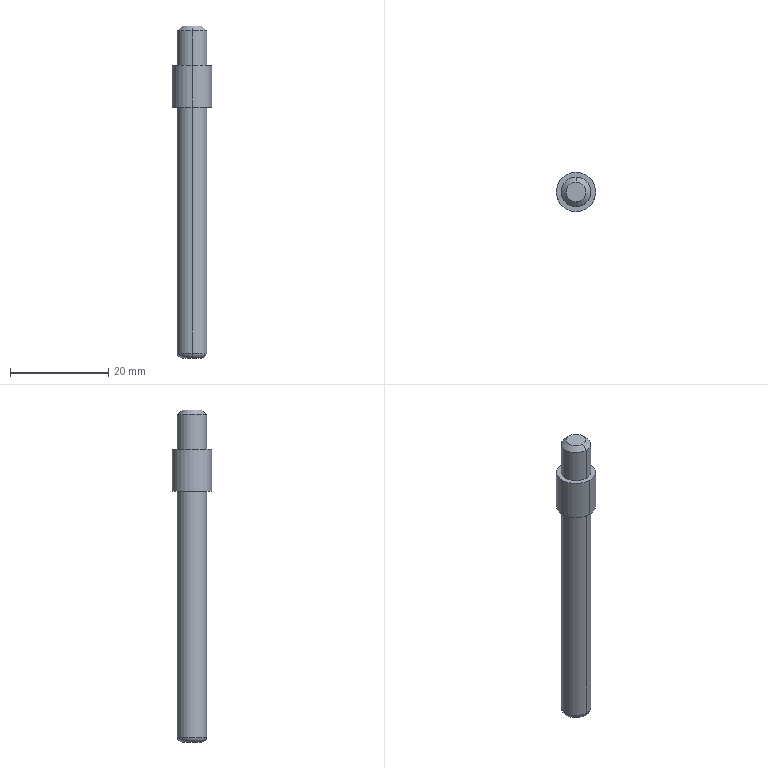Part | SolidWorks | features Chamfer 1, Fillet 1, Revolution 1 | 1 solid | 14 faces | box 8 x 8 x 67.5 mm | volume 2083 mm3 | cylinder 6 | plane 4 | cone 2 | torus 2 | commonest cylinder face diameters 6 x4 8 x2
STEP:
#1=CARTESIAN_POINT('',(0.,-2.,0.));
#2=VERTEX_POINT('',#1);
#3=CARTESIAN_POINT('',(0.,2.,0.));
#4=VERTEX_POINT('',#3);
#5=CARTESIAN_POINT('',(0.,0.,0.));
#6=DIRECTION('',(0.,0.,1.));
#7=DIRECTION('',(0.,-1.,0.));
#8=AXIS2_PLACEMENT_3D('',#5,#6,#7);
#9=CIRCLE('',#8,2.);
#10=EDGE_CURVE('',#2,#4,#9,.T.);
#11=ORIENTED_EDGE('',*,*,#10,.F.);
#12=CARTESIAN_POINT('',(0.,-3.,-1.));
#13=VERTEX_POINT('',#12);
#14=CARTESIAN_POINT('',(0.,-3.,-1.));
#15=DIRECTION('',(0.,-0.7071,-0.7071));
#16=VECTOR('',#15,1000.);
#17=LINE('',#14,#16);
#18=EDGE_CURVE('',#2,#13,#17,.T.);
#19=ORIENTED_EDGE('',*,*,#18,.T.);
#20=CARTESIAN_POINT('',(0.,3.,-1.));
#21=VERTEX_POINT('',#20);
#22=CARTESIAN_POINT('',(0.,0.,-1.));
#23=DIRECTION('',(0.,0.,-1.));
#24=DIRECTION('',(0.,-1.,0.));
#25=AXIS2_PLACEMENT_3D('',#22,#23,#24);
#26=CIRCLE('',#25,3.);
#27=EDGE_CURVE('',#21,#13,#26,.T.);
#28=ORIENTED_EDGE('',*,*,#27,.F.);
#29=CARTESIAN_POINT('',(0.,3.,-1.));
#30=DIRECTION('',(0.,0.7071,-0.7071));
#31=VECTOR('',#30,1000.);
#32=LINE('',#29,#31);
#33=EDGE_CURVE('',#4,#21,#32,.T.);
#34=ORIENTED_EDGE('',*,*,#33,.F.);
#35=EDGE_LOOP('',(#11,#19,#28,#34));
#36=FACE_OUTER_BOUND('',#35,.T.);
#37=CARTESIAN_POINT('',(0.,0.,-1.));
#38=DIRECTION('',(0.,0.,-1.));
#39=DIRECTION('',(0.,1.,0.));
#40=AXIS2_PLACEMENT_3D('',#37,#38,#39);
#41=CONICAL_SURFACE('',#40,3.,0.7854);
#42=ADVANCED_FACE('',(#36),#41,.T.);
#43=CARTESIAN_POINT('',(0.,-3.,-66.5));
#44=VERTEX_POINT('',#43);
#45=CARTESIAN_POINT('',(0.,3.,-66.5));
#46=VERTEX_POINT('',#45);
#47=CARTESIAN_POINT('',(0.,0.,-66.5));
#48=DIRECTION('',(0.,0.,1.));
#49=DIRECTION('',(0.,1.,0.));
#50=AXIS2_PLACEMENT_3D('',#47,#48,#49);
#51=CIRCLE('',#50,3.);
#52=EDGE_CURVE('',#44,#46,#51,.T.);
#53=ORIENTED_EDGE('',*,*,#52,.F.);
#54=CARTESIAN_POINT('',(0.,-2.,-67.5));
#55=VERTEX_POINT('',#54);
#56=CARTESIAN_POINT('',(0.,-2.,-66.5));
#57=DIRECTION('',(1.,0.,0.));
#58=DIRECTION('',(0.,1.,0.));
#59=AXIS2_PLACEMENT_3D('',#56,#57,#58);
#60=CIRCLE('',#59,1.);
#61=EDGE_CURVE('',#44,#55,#60,.T.);
#62=ORIENTED_EDGE('',*,*,#61,.T.);
#63=CARTESIAN_POINT('',(0.,2.,-67.5));
#64=VERTEX_POINT('',#63);
#65=CARTESIAN_POINT('',(0.,0.,-67.5));
#66=DIRECTION('',(0.,0.,-1.));
#67=DIRECTION('',(0.,1.,0.));
#68=AXIS2_PLACEMENT_3D('',#65,#66,#67);
#69=CIRCLE('',#68,2.);
#70=EDGE_CURVE('',#64,#55,#69,.T.);
#71=ORIENTED_EDGE('',*,*,#70,.F.);
#72=CARTESIAN_POINT('',(0.,2.,-66.5));
#73=DIRECTION('',(-1.,0.,0.));
#74=DIRECTION('',(0.,0.,1.));
#75=AXIS2_PLACEMENT_3D('',#72,#73,#74);
#76=CIRCLE('',#75,1.);
#77=EDGE_CURVE('',#46,#64,#76,.T.);
#78=ORIENTED_EDGE('',*,*,#77,.F.);
#79=EDGE_LOOP('',(#53,#62,#71,#78));
#80=FACE_OUTER_BOUND('',#79,.T.);
#81=CARTESIAN_POINT('',(0.,0.,-66.5));
#82=DIRECTION('',(0.,0.,-1.));
#83=DIRECTION('',(0.,1.,0.));
#84=AXIS2_PLACEMENT_3D('',#81,#82,#83);
#85=TOROIDAL_SURFACE('',#84,2.,1.);
#86=ADVANCED_FACE('',(#80),#85,.T.);
#87=CARTESIAN_POINT('',(0.,3.,-16.5));
#88=VERTEX_POINT('',#87);
#89=CARTESIAN_POINT('',(0.,-3.,-16.5));
#90=VERTEX_POINT('',#89);
#91=CARTESIAN_POINT('',(0.,0.,-16.5));
#92=DIRECTION('',(0.,0.,-1.));
#93=DIRECTION('',(0.,1.,0.));
#94=AXIS2_PLACEMENT_3D('',#91,#92,#93);
#95=CIRCLE('',#94,3.);
#96=EDGE_CURVE('',#88,#90,#95,.T.);
#97=ORIENTED_EDGE('',*,*,#96,.T.);
#98=CARTESIAN_POINT('',(0.,-3.,-67.5));
#99=DIRECTION('',(0.,0.,-1.));
#100=VECTOR('',#99,1000.);
#101=LINE('',#98,#100);
#102=EDGE_CURVE('',#90,#44,#101,.T.);
#103=ORIENTED_EDGE('',*,*,#102,.T.);
#104=ORIENTED_EDGE('',*,*,#52,.T.);
#105=CARTESIAN_POINT('',(0.,3.,-67.5));
#106=DIRECTION('',(0.,0.,-1.));
#107=VECTOR('',#106,1000.);
#108=LINE('',#105,#107);
#109=EDGE_CURVE('',#88,#46,#108,.T.);
#110=ORIENTED_EDGE('',*,*,#109,.F.);
#111=EDGE_LOOP('',(#97,#103,#104,#110));
#112=FACE_OUTER_BOUND('',#111,.T.);
#113=CARTESIAN_POINT('',(0.,0.,-67.5));
#114=DIRECTION('',(0.,0.,-1.));
#115=DIRECTION('',(0.,1.,0.));
#116=AXIS2_PLACEMENT_3D('',#113,#114,#115);
#117=CYLINDRICAL_SURFACE('',#116,3.);
#118=ADVANCED_FACE('',(#112),#117,.T.);
#119=CARTESIAN_POINT('',(0.,4.,-8.));
#120=VERTEX_POINT('',#119);
#121=CARTESIAN_POINT('',(0.,-4.,-8.));
#122=VERTEX_POINT('',#121);
#123=CARTESIAN_POINT('',(0.,0.,-8.));
#124=DIRECTION('',(0.,0.,-1.));
#125=DIRECTION('',(0.,1.,0.));
#126=AXIS2_PLACEMENT_3D('',#123,#124,#125);
#127=CIRCLE('',#126,4.);
#128=EDGE_CURVE('',#120,#122,#127,.T.);
#129=ORIENTED_EDGE('',*,*,#128,.T.);
#130=CARTESIAN_POINT('',(0.,-4.,-16.5));
#131=VERTEX_POINT('',#130);
#132=CARTESIAN_POINT('',(0.,-4.,-67.5));
#133=DIRECTION('',(0.,0.,-1.));
#134=VECTOR('',#133,1000.);
#135=LINE('',#132,#134);
#136=EDGE_CURVE('',#122,#131,#135,.T.);
#137=ORIENTED_EDGE('',*,*,#136,.T.);
#138=CARTESIAN_POINT('',(0.,4.,-16.5));
#139=VERTEX_POINT('',#138);
#140=CARTESIAN_POINT('',(0.,0.,-16.5));
#141=DIRECTION('',(0.,0.,-1.));
#142=DIRECTION('',(0.,1.,0.));
#143=AXIS2_PLACEMENT_3D('',#140,#141,#142);
#144=CIRCLE('',#143,4.);
#145=EDGE_CURVE('',#139,#131,#144,.T.);
#146=ORIENTED_EDGE('',*,*,#145,.F.);
#147=CARTESIAN_POINT('',(0.,4.,-67.5));
#148=DIRECTION('',(0.,0.,-1.));
#149=VECTOR('',#148,1000.);
#150=LINE('',#147,#149);
#151=EDGE_CURVE('',#120,#139,#150,.T.);
#152=ORIENTED_EDGE('',*,*,#151,.F.);
#153=EDGE_LOOP('',(#129,#137,#146,#152));
#154=FACE_OUTER_BOUND('',#153,.T.);
#155=CARTESIAN_POINT('',(0.,0.,-67.5));
#156=DIRECTION('',(0.,0.,-1.));
#157=DIRECTION('',(0.,1.,0.));
#158=AXIS2_PLACEMENT_3D('',#155,#156,#157);
#159=CYLINDRICAL_SURFACE('',#158,4.);
#160=ADVANCED_FACE('',(#154),#159,.T.);
#161=ORIENTED_EDGE('',*,*,#27,.T.);
#162=CARTESIAN_POINT('',(0.,-3.,-8.));
#163=VERTEX_POINT('',#162);
#164=CARTESIAN_POINT('',(0.,-3.,-67.5));
#165=DIRECTION('',(0.,0.,-1.));
#166=VECTOR('',#165,1000.);
#167=LINE('',#164,#166);
#168=EDGE_CURVE('',#13,#163,#167,.T.);
#169=ORIENTED_EDGE('',*,*,#168,.T.);
#170=CARTESIAN_POINT('',(0.,3.,-8.));
#171=VERTEX_POINT('',#170);
#172=CARTESIAN_POINT('',(0.,0.,-8.));
#173=DIRECTION('',(0.,0.,-1.));
#174=DIRECTION('',(0.,1.,0.));
#175=AXIS2_PLACEMENT_3D('',#172,#173,#174);
#176=CIRCLE('',#175,3.);
#177=EDGE_CURVE('',#171,#163,#176,.T.);
#178=ORIENTED_EDGE('',*,*,#177,.F.);
#179=CARTESIAN_POINT('',(0.,3.,-67.5));
#180=DIRECTION('',(0.,0.,-1.));
#181=VECTOR('',#180,1000.);
#182=LINE('',#179,#181);
#183=EDGE_CURVE('',#21,#171,#182,.T.);
#184=ORIENTED_EDGE('',*,*,#183,.F.);
#185=EDGE_LOOP('',(#161,#169,#178,#184));
#186=FACE_OUTER_BOUND('',#185,.T.);
#187=CARTESIAN_POINT('',(0.,0.,-67.5));
#188=DIRECTION('',(0.,0.,-1.));
#189=DIRECTION('',(0.,1.,0.));
#190=AXIS2_PLACEMENT_3D('',#187,#188,#189);
#191=CYLINDRICAL_SURFACE('',#190,3.);
#192=ADVANCED_FACE('',(#186),#191,.T.);
#193=CARTESIAN_POINT('',(0.,0.,0.));
#194=DIRECTION('',(0.,0.,1.));
#195=DIRECTION('',(0.,-1.,0.));
#196=AXIS2_PLACEMENT_3D('',#193,#194,#195);
#197=CIRCLE('',#196,2.);
#198=EDGE_CURVE('',#4,#2,#197,.T.);
#199=ORIENTED_EDGE('',*,*,#198,.T.);
#200=ORIENTED_EDGE('',*,*,#10,.T.);
#201=EDGE_LOOP('',(#199,#200));
#202=FACE_OUTER_BOUND('',#201,.T.);
#203=CARTESIAN_POINT('',(0.,0.,0.));
#204=DIRECTION('',(0.,0.,1.));
#205=DIRECTION('',(0.,-1.,0.));
#206=AXIS2_PLACEMENT_3D('',#203,#204,#205);
#207=PLANE('',#206);
#208=ADVANCED_FACE('',(#202),#207,.T.);
#209=ORIENTED_EDGE('',*,*,#168,.F.);
#210=CARTESIAN_POINT('',(0.,0.,-1.));
#211=DIRECTION('',(0.,0.,-1.));
#212=DIRECTION('',(0.,-1.,0.));
#213=AXIS2_PLACEMENT_3D('',#210,#211,#212);
#214=CIRCLE('',#213,3.);
#215=EDGE_CURVE('',#13,#21,#214,.T.);
#216=ORIENTED_EDGE('',*,*,#215,.T.);
#217=ORIENTED_EDGE('',*,*,#183,.T.);
#218=CARTESIAN_POINT('',(0.,0.,-8.));
#219=DIRECTION('',(0.,0.,-1.));
#220=DIRECTION('',(0.,1.,0.));
#221=AXIS2_PLACEMENT_3D('',#218,#219,#220);
#222=CIRCLE('',#221,3.);
#223=EDGE_CURVE('',#163,#171,#222,.T.);
#224=ORIENTED_EDGE('',*,*,#223,.F.);
#225=EDGE_LOOP('',(#209,#216,#217,#224));
#226=FACE_OUTER_BOUND('',#225,.T.);
#227=CARTESIAN_POINT('',(0.,0.,-67.5));
#228=DIRECTION('',(0.,0.,-1.));
#229=DIRECTION('',(0.,1.,0.));
#230=AXIS2_PLACEMENT_3D('',#227,#228,#229);
#231=CYLINDRICAL_SURFACE('',#230,3.);
#232=ADVANCED_FACE('',(#226),#231,.T.);
#233=ORIENTED_EDGE('',*,*,#177,.T.);
#234=ORIENTED_EDGE('',*,*,#223,.T.);
#235=EDGE_LOOP('',(#233,#234));
#236=FACE_BOUND('',#235,.T.);
#237=ORIENTED_EDGE('',*,*,#128,.F.);
#238=CARTESIAN_POINT('',(0.,0.,-8.));
#239=DIRECTION('',(0.,0.,-1.));
#240=DIRECTION('',(0.,1.,0.));
#241=AXIS2_PLACEMENT_3D('',#238,#239,#240);
#242=CIRCLE('',#241,4.);
#243=EDGE_CURVE('',#122,#120,#242,.T.);
#244=ORIENTED_EDGE('',*,*,#243,.F.);
#245=EDGE_LOOP('',(#237,#244));
#246=FACE_OUTER_BOUND('',#245,.T.);
#247=CARTESIAN_POINT('',(0.,3.,-8.));
#248=DIRECTION('',(0.,0.,1.));
#249=DIRECTION('',(0.,-1.,0.));
#250=AXIS2_PLACEMENT_3D('',#247,#248,#249);
#251=PLANE('',#250);
#252=ADVANCED_FACE('',(#236,#246),#251,.T.);
#253=ORIENTED_EDGE('',*,*,#136,.F.);
#254=ORIENTED_EDGE('',*,*,#243,.T.);
#255=ORIENTED_EDGE('',*,*,#151,.T.);
#256=CARTESIAN_POINT('',(0.,0.,-16.5));
#257=DIRECTION('',(0.,0.,-1.));
#258=DIRECTION('',(0.,1.,0.));
#259=AXIS2_PLACEMENT_3D('',#256,#257,#258);
#260=CIRCLE('',#259,4.);
#261=EDGE_CURVE('',#131,#139,#260,.T.);
#262=ORIENTED_EDGE('',*,*,#261,.F.);
#263=EDGE_LOOP('',(#253,#254,#255,#262));
#264=FACE_OUTER_BOUND('',#263,.T.);
#265=CARTESIAN_POINT('',(0.,0.,-67.5));
#266=DIRECTION('',(0.,0.,-1.));
#267=DIRECTION('',(0.,1.,0.));
#268=AXIS2_PLACEMENT_3D('',#265,#266,#267);
#269=CYLINDRICAL_SURFACE('',#268,4.);
#270=ADVANCED_FACE('',(#264),#269,.T.);
#271=ORIENTED_EDGE('',*,*,#145,.T.);
#272=ORIENTED_EDGE('',*,*,#261,.T.);
#273=EDGE_LOOP('',(#271,#272));
#274=FACE_OUTER_BOUND('',#273,.T.);
#275=ORIENTED_EDGE('',*,*,#96,.F.);
#276=CARTESIAN_POINT('',(0.,0.,-16.5));
#277=DIRECTION('',(0.,0.,-1.));
#278=DIRECTION('',(0.,1.,0.));
#279=AXIS2_PLACEMENT_3D('',#276,#277,#278);
#280=CIRCLE('',#279,3.);
#281=EDGE_CURVE('',#90,#88,#280,.T.);
#282=ORIENTED_EDGE('',*,*,#281,.F.);
#283=EDGE_LOOP('',(#275,#282));
#284=FACE_BOUND('',#283,.T.);
#285=CARTESIAN_POINT('',(0.,4.,-16.5));
#286=DIRECTION('',(0.,0.,-1.));
#287=DIRECTION('',(0.,1.,0.));
#288=AXIS2_PLACEMENT_3D('',#285,#286,#287);
#289=PLANE('',#288);
#290=ADVANCED_FACE('',(#274,#284),#289,.T.);
#291=ORIENTED_EDGE('',*,*,#102,.F.);
#292=ORIENTED_EDGE('',*,*,#281,.T.);
#293=ORIENTED_EDGE('',*,*,#109,.T.);
#294=CARTESIAN_POINT('',(0.,0.,-66.5));
#295=DIRECTION('',(0.,0.,1.));
#296=DIRECTION('',(0.,1.,0.));
#297=AXIS2_PLACEMENT_3D('',#294,#295,#296);
#298=CIRCLE('',#297,3.);
#299=EDGE_CURVE('',#46,#44,#298,.T.);
#300=ORIENTED_EDGE('',*,*,#299,.T.);
#301=EDGE_LOOP('',(#291,#292,#293,#300));
#302=FACE_OUTER_BOUND('',#301,.T.);
#303=CARTESIAN_POINT('',(0.,0.,-67.5));
#304=DIRECTION('',(0.,0.,-1.));
#305=DIRECTION('',(0.,1.,0.));
#306=AXIS2_PLACEMENT_3D('',#303,#304,#305);
#307=CYLINDRICAL_SURFACE('',#306,3.);
#308=ADVANCED_FACE('',(#302),#307,.T.);
#309=ORIENTED_EDGE('',*,*,#70,.T.);
#310=CARTESIAN_POINT('',(0.,0.,-67.5));
#311=DIRECTION('',(0.,0.,-1.));
#312=DIRECTION('',(0.,1.,0.));
#313=AXIS2_PLACEMENT_3D('',#310,#311,#312);
#314=CIRCLE('',#313,2.);
#315=EDGE_CURVE('',#55,#64,#314,.T.);
#316=ORIENTED_EDGE('',*,*,#315,.T.);
#317=EDGE_LOOP('',(#309,#316));
#318=FACE_OUTER_BOUND('',#317,.T.);
#319=CARTESIAN_POINT('',(0.,3.,-67.5));
#320=DIRECTION('',(0.,0.,-1.));
#321=DIRECTION('',(0.,1.,0.));
#322=AXIS2_PLACEMENT_3D('',#319,#320,#321);
#323=PLANE('',#322);
#324=ADVANCED_FACE('',(#318),#323,.T.);
#325=ORIENTED_EDGE('',*,*,#61,.F.);
#326=ORIENTED_EDGE('',*,*,#299,.F.);
#327=ORIENTED_EDGE('',*,*,#77,.T.);
#328=ORIENTED_EDGE('',*,*,#315,.F.);
#329=EDGE_LOOP('',(#325,#326,#327,#328));
#330=FACE_OUTER_BOUND('',#329,.T.);
#331=CARTESIAN_POINT('',(0.,0.,-66.5));
#332=DIRECTION('',(0.,0.,-1.));
#333=DIRECTION('',(0.,1.,0.));
#334=AXIS2_PLACEMENT_3D('',#331,#332,#333);
#335=TOROIDAL_SURFACE('',#334,2.,1.);
#336=ADVANCED_FACE('',(#330),#335,.T.);
#337=ORIENTED_EDGE('',*,*,#18,.F.);
#338=ORIENTED_EDGE('',*,*,#198,.F.);
#339=ORIENTED_EDGE('',*,*,#33,.T.);
#340=ORIENTED_EDGE('',*,*,#215,.F.);
#341=EDGE_LOOP('',(#337,#338,#339,#340));
#342=FACE_OUTER_BOUND('',#341,.T.);
#343=CARTESIAN_POINT('',(0.,0.,-1.));
#344=DIRECTION('',(0.,0.,-1.));
#345=DIRECTION('',(0.,1.,0.));
#346=AXIS2_PLACEMENT_3D('',#343,#344,#345);
#347=CONICAL_SURFACE('',#346,3.,0.7854);
#348=ADVANCED_FACE('',(#342),#347,.T.);
#349=CLOSED_SHELL('',(#42,#86,#118,#160,#192,#208,#232,#252,#270,#290,#308,#324,#336,#348));
#350=MANIFOLD_SOLID_BREP('',#349);
#351=CARTESIAN_POINT('',(0.,0.,0.));
#352=DIRECTION('',(0.,0.,1.));
#353=DIRECTION('',(1.,0.,0.));
#354=AXIS2_PLACEMENT_3D('',#351,#352,#353);
#355=(LENGTH_UNIT()NAMED_UNIT(*)SI_UNIT(.MILLI.,.METRE.));
#356=UNCERTAINTY_MEASURE_WITH_UNIT(LENGTH_MEASURE(0.00001),#355,'','');
#357=(NAMED_UNIT(*)PLANE_ANGLE_UNIT()SI_UNIT($,.RADIAN.));
#358=(NAMED_UNIT(*)SI_UNIT($,.STERADIAN.)SOLID_ANGLE_UNIT());
#359=(GEOMETRIC_REPRESENTATION_CONTEXT(3)GLOBAL_UNCERTAINTY_ASSIGNED_CONTEXT((#356))GLOBAL_UNIT_ASSIGNED_CONTEXT((#355,#357,#358))REPRESENTATION_CONTEXT('',''));
#360=ADVANCED_BREP_SHAPE_REPRESENTATION('',(#350,#354),#359);